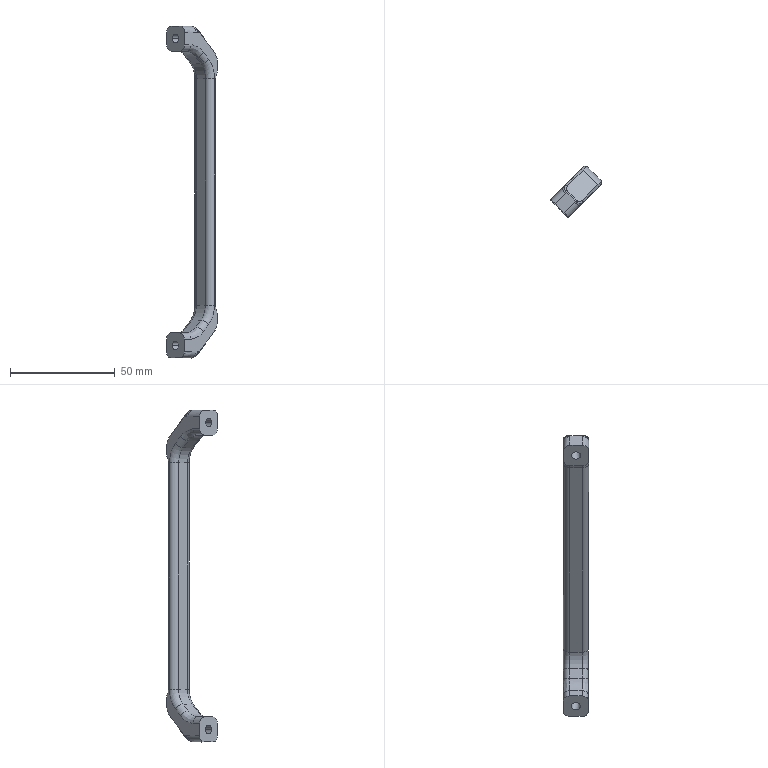Part | SolidWorks | features BaseBody 1 | 1 solid | 100 faces | box 24.389 x 24.336 x 158.808 mm | volume 13231 mm3 | cylinder 42 | plane 26 | spline 20 | cone 8 | torus 4 | commonest cylinder face diameters 6 x26 20 x6 4.2 x4 10 x4 16 x2